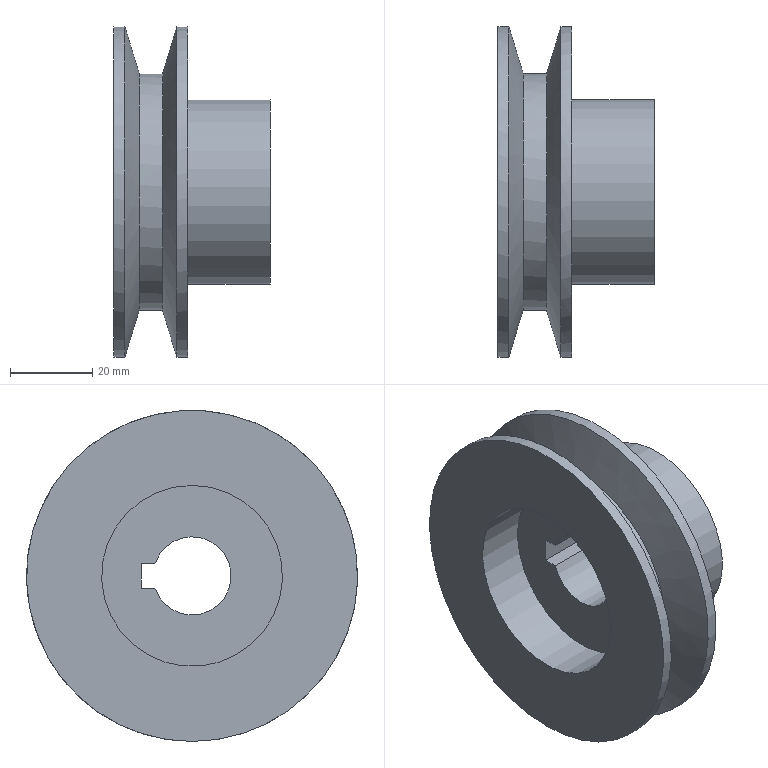Part | STEP file | Plain V-belt pulley_solid wheel_A75X16X1X38X45 | 1 solid | 15 faces | box 38 x 80.5 x 80.5 mm | volume 74057 mm3 | plane 7 | cylinder 6 | cone 2 | commonest cylinder face diameters 80.5 x2 19 x1 44 x1 45 x1 57.6 x1
STEP:
#1=CARTESIAN_POINT('',(0.,0.,0.));
#2=DIRECTION('',(0.,0.,1.));
#3=DIRECTION('',(1.,0.,0.));
#4=AXIS2_PLACEMENT_3D('',#1,#2,#3);
#5=CARTESIAN_POINT('',(12.,9.014,-3.));
#6=VERTEX_POINT('',#5);
#7=CARTESIAN_POINT('',(12.,12.3,-3.));
#8=VERTEX_POINT('',#7);
#9=CARTESIAN_POINT('',(12.,12.3,-3.));
#10=DIRECTION('',(0.,1.,0.));
#11=VECTOR('',#10,1.);
#12=LINE('',#9,#11);
#13=CARTESIAN_POINT('',(38.,12.3,-3.));
#14=DIRECTION('',(0.,0.,-1.));
#15=DIRECTION('',(0.,1.,0.));
#16=AXIS2_PLACEMENT_3D('',#13,#14,#15);
#17=PLANE('',#16);
#18=CARTESIAN_POINT('',(0.,-26.));
#19=DIRECTION('',(1.,0.));
#20=VECTOR('',#19,1.);
#21=LINE('',#18,#20);
#22=(GEOMETRIC_REPRESENTATION_CONTEXT(2)PARAMETRIC_REPRESENTATION_CONTEXT()REPRESENTATION_CONTEXT('',''));
#23=DEFINITIONAL_REPRESENTATION('',(#21),#22);
#24=PCURVE('',#17,#23);
#25=CARTESIAN_POINT('',(12.,0.,0.));
#26=DIRECTION('',(-1.,0.,0.));
#27=DIRECTION('',(0.,0.,1.));
#28=AXIS2_PLACEMENT_3D('',#25,#26,#27);
#29=PLANE('',#28);
#30=CARTESIAN_POINT('',(-3.,12.3));
#31=DIRECTION('',(0.,1.));
#32=VECTOR('',#31,1.);
#33=LINE('',#30,#32);
#34=(GEOMETRIC_REPRESENTATION_CONTEXT(2)PARAMETRIC_REPRESENTATION_CONTEXT()REPRESENTATION_CONTEXT('',''));
#35=DEFINITIONAL_REPRESENTATION('',(#33),#34);
#36=PCURVE('',#29,#35);
#37=SURFACE_CURVE('',#12,(#24,#36),.PCURVE_S1.);
#38=EDGE_CURVE('',#6,#8,#37,.T.);
#39=ORIENTED_EDGE('',*,*,#38,.F.);
#40=CARTESIAN_POINT('',(38.,9.014,-3.));
#41=VERTEX_POINT('',#40);
#42=CARTESIAN_POINT('',(38.,9.014,-3.));
#43=DIRECTION('',(-1.,0.,0.));
#44=VECTOR('',#43,1.);
#45=LINE('',#42,#44);
#46=CARTESIAN_POINT('',(-3.286,0.));
#47=DIRECTION('',(0.,-1.));
#48=VECTOR('',#47,1.);
#49=LINE('',#46,#48);
#50=(GEOMETRIC_REPRESENTATION_CONTEXT(2)PARAMETRIC_REPRESENTATION_CONTEXT()REPRESENTATION_CONTEXT('',''));
#51=DEFINITIONAL_REPRESENTATION('',(#49),#50);
#52=PCURVE('',#17,#51);
#53=CARTESIAN_POINT('',(38.,0.,0.));
#54=DIRECTION('',(-1.,0.,0.));
#55=DIRECTION('',(0.,0.,1.));
#56=AXIS2_PLACEMENT_3D('',#53,#54,#55);
#57=CYLINDRICAL_SURFACE('',#56,9.5);
#58=CARTESIAN_POINT('',(1.892,0.));
#59=DIRECTION('',(0.,1.));
#60=VECTOR('',#59,1.);
#61=LINE('',#58,#60);
#62=(GEOMETRIC_REPRESENTATION_CONTEXT(2)PARAMETRIC_REPRESENTATION_CONTEXT()REPRESENTATION_CONTEXT('',''));
#63=DEFINITIONAL_REPRESENTATION('',(#61),#62);
#64=PCURVE('',#57,#63);
#65=SURFACE_CURVE('',#45,(#52,#64),.PCURVE_S1.);
#66=EDGE_CURVE('',#41,#6,#65,.T.);
#67=ORIENTED_EDGE('',*,*,#66,.F.);
#68=CARTESIAN_POINT('',(38.,12.3,-3.));
#69=VERTEX_POINT('',#68);
#70=CARTESIAN_POINT('',(38.,12.3,-3.));
#71=DIRECTION('',(0.,-1.,0.));
#72=VECTOR('',#71,1.);
#73=LINE('',#70,#72);
#74=CARTESIAN_POINT('',(0.,0.));
#75=DIRECTION('',(-1.,0.));
#76=VECTOR('',#75,1.);
#77=LINE('',#74,#76);
#78=(GEOMETRIC_REPRESENTATION_CONTEXT(2)PARAMETRIC_REPRESENTATION_CONTEXT()REPRESENTATION_CONTEXT('',''));
#79=DEFINITIONAL_REPRESENTATION('',(#77),#78);
#80=PCURVE('',#17,#79);
#81=CARTESIAN_POINT('',(38.,15.25,0.));
#82=DIRECTION('',(1.,0.,0.));
#83=DIRECTION('',(0.,0.,-1.));
#84=AXIS2_PLACEMENT_3D('',#81,#82,#83);
#85=PLANE('',#84);
#86=CARTESIAN_POINT('',(3.,-2.95));
#87=DIRECTION('',(0.,-1.));
#88=VECTOR('',#87,1.);
#89=LINE('',#86,#88);
#90=(GEOMETRIC_REPRESENTATION_CONTEXT(2)PARAMETRIC_REPRESENTATION_CONTEXT()REPRESENTATION_CONTEXT('',''));
#91=DEFINITIONAL_REPRESENTATION('',(#89),#90);
#92=PCURVE('',#85,#91);
#93=SURFACE_CURVE('',#73,(#80,#92),.PCURVE_S1.);
#94=EDGE_CURVE('',#69,#41,#93,.T.);
#95=ORIENTED_EDGE('',*,*,#94,.F.);
#96=CARTESIAN_POINT('',(38.,12.3,-3.));
#97=DIRECTION('',(-1.,0.,0.));
#98=VECTOR('',#97,1.);
#99=LINE('',#96,#98);
#100=CARTESIAN_POINT('',(0.,0.));
#101=DIRECTION('',(0.,-1.));
#102=VECTOR('',#101,1.);
#103=LINE('',#100,#102);
#104=(GEOMETRIC_REPRESENTATION_CONTEXT(2)PARAMETRIC_REPRESENTATION_CONTEXT()REPRESENTATION_CONTEXT('',''));
#105=DEFINITIONAL_REPRESENTATION('',(#103),#104);
#106=PCURVE('',#17,#105);
#107=CARTESIAN_POINT('',(38.,12.3,-3.));
#108=DIRECTION('',(0.,1.,0.));
#109=DIRECTION('',(0.,0.,1.));
#110=AXIS2_PLACEMENT_3D('',#107,#108,#109);
#111=PLANE('',#110);
#112=CARTESIAN_POINT('',(0.,0.));
#113=DIRECTION('',(0.,-1.));
#114=VECTOR('',#113,1.);
#115=LINE('',#112,#114);
#116=(GEOMETRIC_REPRESENTATION_CONTEXT(2)PARAMETRIC_REPRESENTATION_CONTEXT()REPRESENTATION_CONTEXT('',''));
#117=DEFINITIONAL_REPRESENTATION('',(#115),#116);
#118=PCURVE('',#111,#117);
#119=SURFACE_CURVE('',#99,(#106,#118),.PCURVE_S1.);
#120=EDGE_CURVE('',#69,#8,#119,.T.);
#121=ORIENTED_EDGE('',*,*,#120,.T.);
#122=EDGE_LOOP('',(#39,#67,#95,#121));
#123=FACE_BOUND('',#122,.T.);
#124=ADVANCED_FACE('',(#123),#17,.F.);
#125=CARTESIAN_POINT('',(12.,12.3,3.));
#126=VERTEX_POINT('',#125);
#127=CARTESIAN_POINT('',(12.,12.3,-3.));
#128=DIRECTION('',(0.,0.,1.));
#129=VECTOR('',#128,1.);
#130=LINE('',#127,#129);
#131=CARTESIAN_POINT('',(0.,-26.));
#132=DIRECTION('',(1.,0.));
#133=VECTOR('',#132,1.);
#134=LINE('',#131,#133);
#135=(GEOMETRIC_REPRESENTATION_CONTEXT(2)PARAMETRIC_REPRESENTATION_CONTEXT()REPRESENTATION_CONTEXT('',''));
#136=DEFINITIONAL_REPRESENTATION('',(#134),#135);
#137=PCURVE('',#111,#136);
#138=CARTESIAN_POINT('',(-3.,12.3));
#139=DIRECTION('',(1.,0.));
#140=VECTOR('',#139,1.);
#141=LINE('',#138,#140);
#142=(GEOMETRIC_REPRESENTATION_CONTEXT(2)PARAMETRIC_REPRESENTATION_CONTEXT()REPRESENTATION_CONTEXT('',''));
#143=DEFINITIONAL_REPRESENTATION('',(#141),#142);
#144=PCURVE('',#29,#143);
#145=SURFACE_CURVE('',#130,(#137,#144),.PCURVE_S1.);
#146=EDGE_CURVE('',#8,#126,#145,.T.);
#147=ORIENTED_EDGE('',*,*,#146,.F.);
#148=ORIENTED_EDGE('',*,*,#120,.F.);
#149=CARTESIAN_POINT('',(38.,12.3,3.));
#150=VERTEX_POINT('',#149);
#151=CARTESIAN_POINT('',(38.,12.3,-3.));
#152=DIRECTION('',(0.,0.,-1.));
#153=VECTOR('',#152,1.);
#154=LINE('',#151,#153);
#155=CARTESIAN_POINT('',(0.,0.));
#156=DIRECTION('',(-1.,0.));
#157=VECTOR('',#156,1.);
#158=LINE('',#155,#157);
#159=(GEOMETRIC_REPRESENTATION_CONTEXT(2)PARAMETRIC_REPRESENTATION_CONTEXT()REPRESENTATION_CONTEXT('',''));
#160=DEFINITIONAL_REPRESENTATION('',(#158),#159);
#161=PCURVE('',#111,#160);
#162=CARTESIAN_POINT('',(3.,-2.95));
#163=DIRECTION('',(1.,0.));
#164=VECTOR('',#163,1.);
#165=LINE('',#162,#164);
#166=(GEOMETRIC_REPRESENTATION_CONTEXT(2)PARAMETRIC_REPRESENTATION_CONTEXT()REPRESENTATION_CONTEXT('',''));
#167=DEFINITIONAL_REPRESENTATION('',(#165),#166);
#168=PCURVE('',#85,#167);
#169=SURFACE_CURVE('',#154,(#161,#168),.PCURVE_S1.);
#170=EDGE_CURVE('',#150,#69,#169,.T.);
#171=ORIENTED_EDGE('',*,*,#170,.F.);
#172=CARTESIAN_POINT('',(38.,12.3,3.));
#173=DIRECTION('',(-1.,0.,0.));
#174=VECTOR('',#173,1.);
#175=LINE('',#172,#174);
#176=CARTESIAN_POINT('',(6.,0.));
#177=DIRECTION('',(0.,-1.));
#178=VECTOR('',#177,1.);
#179=LINE('',#176,#178);
#180=(GEOMETRIC_REPRESENTATION_CONTEXT(2)PARAMETRIC_REPRESENTATION_CONTEXT()REPRESENTATION_CONTEXT('',''));
#181=DEFINITIONAL_REPRESENTATION('',(#179),#180);
#182=PCURVE('',#111,#181);
#183=CARTESIAN_POINT('',(38.,12.3,3.));
#184=DIRECTION('',(0.,0.,1.));
#185=DIRECTION('',(1.,0.,0.));
#186=AXIS2_PLACEMENT_3D('',#183,#184,#185);
#187=PLANE('',#186);
#188=CARTESIAN_POINT('',(0.,0.));
#189=DIRECTION('',(-1.,0.));
#190=VECTOR('',#189,1.);
#191=LINE('',#188,#190);
#192=(GEOMETRIC_REPRESENTATION_CONTEXT(2)PARAMETRIC_REPRESENTATION_CONTEXT()REPRESENTATION_CONTEXT('',''));
#193=DEFINITIONAL_REPRESENTATION('',(#191),#192);
#194=PCURVE('',#187,#193);
#195=SURFACE_CURVE('',#175,(#182,#194),.PCURVE_S1.);
#196=EDGE_CURVE('',#150,#126,#195,.T.);
#197=ORIENTED_EDGE('',*,*,#196,.T.);
#198=EDGE_LOOP('',(#147,#148,#171,#197));
#199=FACE_BOUND('',#198,.T.);
#200=ADVANCED_FACE('',(#199),#111,.F.);
#201=CARTESIAN_POINT('',(12.,9.014,3.));
#202=VERTEX_POINT('',#201);
#203=CARTESIAN_POINT('',(12.,12.3,3.));
#204=DIRECTION('',(0.,-1.,0.));
#205=VECTOR('',#204,1.);
#206=LINE('',#203,#205);
#207=CARTESIAN_POINT('',(-26.,0.));
#208=DIRECTION('',(0.,-1.));
#209=VECTOR('',#208,1.);
#210=LINE('',#207,#209);
#211=(GEOMETRIC_REPRESENTATION_CONTEXT(2)PARAMETRIC_REPRESENTATION_CONTEXT()REPRESENTATION_CONTEXT('',''));
#212=DEFINITIONAL_REPRESENTATION('',(#210),#211);
#213=PCURVE('',#187,#212);
#214=CARTESIAN_POINT('',(3.,12.3));
#215=DIRECTION('',(0.,-1.));
#216=VECTOR('',#215,1.);
#217=LINE('',#214,#216);
#218=(GEOMETRIC_REPRESENTATION_CONTEXT(2)PARAMETRIC_REPRESENTATION_CONTEXT()REPRESENTATION_CONTEXT('',''));
#219=DEFINITIONAL_REPRESENTATION('',(#217),#218);
#220=PCURVE('',#29,#219);
#221=SURFACE_CURVE('',#206,(#213,#220),.PCURVE_S1.);
#222=EDGE_CURVE('',#126,#202,#221,.T.);
#223=ORIENTED_EDGE('',*,*,#222,.F.);
#224=ORIENTED_EDGE('',*,*,#196,.F.);
#225=CARTESIAN_POINT('',(38.,9.014,3.));
#226=VERTEX_POINT('',#225);
#227=CARTESIAN_POINT('',(38.,12.3,3.));
#228=DIRECTION('',(0.,1.,0.));
#229=VECTOR('',#228,1.);
#230=LINE('',#227,#229);
#231=CARTESIAN_POINT('',(0.,0.));
#232=DIRECTION('',(0.,1.));
#233=VECTOR('',#232,1.);
#234=LINE('',#231,#233);
#235=(GEOMETRIC_REPRESENTATION_CONTEXT(2)PARAMETRIC_REPRESENTATION_CONTEXT()REPRESENTATION_CONTEXT('',''));
#236=DEFINITIONAL_REPRESENTATION('',(#234),#235);
#237=PCURVE('',#187,#236);
#238=CARTESIAN_POINT('',(-3.,-2.95));
#239=DIRECTION('',(0.,1.));
#240=VECTOR('',#239,1.);
#241=LINE('',#238,#240);
#242=(GEOMETRIC_REPRESENTATION_CONTEXT(2)PARAMETRIC_REPRESENTATION_CONTEXT()REPRESENTATION_CONTEXT('',''));
#243=DEFINITIONAL_REPRESENTATION('',(#241),#242);
#244=PCURVE('',#85,#243);
#245=SURFACE_CURVE('',#230,(#237,#244),.PCURVE_S1.);
#246=EDGE_CURVE('',#226,#150,#245,.T.);
#247=ORIENTED_EDGE('',*,*,#246,.F.);
#248=CARTESIAN_POINT('',(38.,9.014,3.));
#249=DIRECTION('',(-1.,0.,0.));
#250=VECTOR('',#249,1.);
#251=LINE('',#248,#250);
#252=CARTESIAN_POINT('',(0.,-3.286));
#253=DIRECTION('',(-1.,0.));
#254=VECTOR('',#253,1.);
#255=LINE('',#252,#254);
#256=(GEOMETRIC_REPRESENTATION_CONTEXT(2)PARAMETRIC_REPRESENTATION_CONTEXT()REPRESENTATION_CONTEXT('',''));
#257=DEFINITIONAL_REPRESENTATION('',(#255),#256);
#258=PCURVE('',#187,#257);
#259=CARTESIAN_POINT('',(7.533,0.));
#260=DIRECTION('',(0.,1.));
#261=VECTOR('',#260,1.);
#262=LINE('',#259,#261);
#263=(GEOMETRIC_REPRESENTATION_CONTEXT(2)PARAMETRIC_REPRESENTATION_CONTEXT()REPRESENTATION_CONTEXT('',''));
#264=DEFINITIONAL_REPRESENTATION('',(#262),#263);
#265=PCURVE('',#57,#264);
#266=SURFACE_CURVE('',#251,(#258,#265),.PCURVE_S1.);
#267=EDGE_CURVE('',#226,#202,#266,.T.);
#268=ORIENTED_EDGE('',*,*,#267,.T.);
#269=EDGE_LOOP('',(#223,#224,#247,#268));
#270=FACE_BOUND('',#269,.T.);
#271=ADVANCED_FACE('',(#270),#187,.F.);
#272=ORIENTED_EDGE('',*,*,#66,.F.);
#273=CARTESIAN_POINT('',(38.,0.,0.));
#274=DIRECTION('',(-1.,0.,0.));
#275=DIRECTION('',(0.,0.,1.));
#276=AXIS2_PLACEMENT_3D('',#273,#274,#275);
#277=CIRCLE('',#276,9.5);
#278=CARTESIAN_POINT('',(0.,0.));
#279=DIRECTION('',(1.,0.));
#280=VECTOR('',#279,1.);
#281=LINE('',#278,#280);
#282=(GEOMETRIC_REPRESENTATION_CONTEXT(2)PARAMETRIC_REPRESENTATION_CONTEXT()REPRESENTATION_CONTEXT('',''));
#283=DEFINITIONAL_REPRESENTATION('',(#281),#282);
#284=PCURVE('',#57,#283);
#285=CARTESIAN_POINT('',(-9.5,-15.25));
#286=CARTESIAN_POINT('',(-9.5,1.204));
#287=CARTESIAN_POINT('',(4.75,-7.023));
#288=CARTESIAN_POINT('',(19.,-15.25));
#289=CARTESIAN_POINT('',(4.75,-23.477));
#290=CARTESIAN_POINT('',(-9.5,-31.704));
#291=CARTESIAN_POINT('',(-9.5,-15.25));
#292=(BOUNDED_CURVE()B_SPLINE_CURVE(2,(#285,#286,#287,#288,#289,#290,#291),.UNSPECIFIED.,.T.,.F.)B_SPLINE_CURVE_WITH_KNOTS((1,2,2,2,2,1),(-2.094,0.,2.094,4.189,6.283,8.378),.UNSPECIFIED.)CURVE()GEOMETRIC_REPRESENTATION_ITEM()RATIONAL_B_SPLINE_CURVE((1.,0.5,1.,0.5,1.,0.5,1.))REPRESENTATION_ITEM(''));
#293=(GEOMETRIC_REPRESENTATION_CONTEXT(2)PARAMETRIC_REPRESENTATION_CONTEXT()REPRESENTATION_CONTEXT('',''));
#294=DEFINITIONAL_REPRESENTATION('',(#292),#293);
#295=PCURVE('',#85,#294);
#296=SURFACE_CURVE('',#277,(#284,#295),.PCURVE_S1.);
#297=EDGE_CURVE('',#41,#226,#296,.T.);
#298=ORIENTED_EDGE('',*,*,#297,.T.);
#299=ORIENTED_EDGE('',*,*,#267,.T.);
#300=CARTESIAN_POINT('',(12.,0.,0.));
#301=DIRECTION('',(1.,0.,0.));
#302=DIRECTION('',(0.,0.,1.));
#303=AXIS2_PLACEMENT_3D('',#300,#301,#302);
#304=CIRCLE('',#303,9.5);
#305=CARTESIAN_POINT('',(12.566,26.));
#306=DIRECTION('',(-1.,0.));
#307=VECTOR('',#306,1.);
#308=LINE('',#305,#307);
#309=(GEOMETRIC_REPRESENTATION_CONTEXT(2)PARAMETRIC_REPRESENTATION_CONTEXT()REPRESENTATION_CONTEXT('',''));
#310=DEFINITIONAL_REPRESENTATION('',(#308),#309);
#311=PCURVE('',#57,#310);
#312=CARTESIAN_POINT('',(9.5,0.));
#313=CARTESIAN_POINT('',(9.5,-16.454));
#314=CARTESIAN_POINT('',(-4.75,-8.227));
#315=CARTESIAN_POINT('',(-19.,0.));
#316=CARTESIAN_POINT('',(-4.75,8.227));
#317=CARTESIAN_POINT('',(9.5,16.454));
#318=CARTESIAN_POINT('',(9.5,0.));
#319=(BOUNDED_CURVE()B_SPLINE_CURVE(2,(#312,#313,#314,#315,#316,#317,#318),.UNSPECIFIED.,.T.,.F.)B_SPLINE_CURVE_WITH_KNOTS((1,2,2,2,2,1),(-2.094,0.,2.094,4.189,6.283,8.378),.UNSPECIFIED.)CURVE()GEOMETRIC_REPRESENTATION_ITEM()RATIONAL_B_SPLINE_CURVE((1.,0.5,1.,0.5,1.,0.5,1.))REPRESENTATION_ITEM(''));
#320=(GEOMETRIC_REPRESENTATION_CONTEXT(2)PARAMETRIC_REPRESENTATION_CONTEXT()REPRESENTATION_CONTEXT('',''));
#321=DEFINITIONAL_REPRESENTATION('',(#319),#320);
#322=PCURVE('',#29,#321);
#323=SURFACE_CURVE('',#304,(#311,#322),.PCURVE_S1.);
#324=EDGE_CURVE('',#202,#6,#323,.T.);
#325=ORIENTED_EDGE('',*,*,#324,.T.);
#326=EDGE_LOOP('',(#272,#298,#299,#325));
#327=FACE_BOUND('',#326,.F.);
#328=ADVANCED_FACE('',(#327),#57,.F.);
#329=CARTESIAN_POINT('',(0.,0.,22.));
#330=VERTEX_POINT('',#329);
#331=CARTESIAN_POINT('',(0.,0.,0.));
#332=DIRECTION('',(-1.,0.,0.));
#333=DIRECTION('',(0.,0.,1.));
#334=AXIS2_PLACEMENT_3D('',#331,#332,#333);
#335=CIRCLE('',#334,22.);
#336=CARTESIAN_POINT('',(0.,31.375,0.));
#337=DIRECTION('',(-1.,0.,0.));
#338=DIRECTION('',(0.,0.,1.));
#339=AXIS2_PLACEMENT_3D('',#336,#337,#338);
#340=PLANE('',#339);
#341=CARTESIAN_POINT('',(0.,-31.375));
#342=DIRECTION('',(1.,0.));
#343=AXIS2_PLACEMENT_2D('',#341,#342);
#344=CIRCLE('',#343,22.);
#345=(GEOMETRIC_REPRESENTATION_CONTEXT(2)PARAMETRIC_REPRESENTATION_CONTEXT()REPRESENTATION_CONTEXT('',''));
#346=DEFINITIONAL_REPRESENTATION('',(#344),#345);
#347=PCURVE('',#340,#346);
#348=CARTESIAN_POINT('',(12.,0.,0.));
#349=DIRECTION('',(-1.,0.,0.));
#350=DIRECTION('',(0.,0.,1.));
#351=AXIS2_PLACEMENT_3D('',#348,#349,#350);
#352=CYLINDRICAL_SURFACE('',#351,22.);
#353=CARTESIAN_POINT('',(0.,12.));
#354=DIRECTION('',(1.,0.));
#355=VECTOR('',#354,1.);
#356=LINE('',#353,#355);
#357=(GEOMETRIC_REPRESENTATION_CONTEXT(2)PARAMETRIC_REPRESENTATION_CONTEXT()REPRESENTATION_CONTEXT('',''));
#358=DEFINITIONAL_REPRESENTATION('',(#356),#357);
#359=PCURVE('',#352,#358);
#360=SURFACE_CURVE('',#335,(#347,#359),.PCURVE_S1.);
#361=EDGE_CURVE('',#330,#330,#360,.T.);
#362=ORIENTED_EDGE('',*,*,#361,.F.);
#363=EDGE_LOOP('',(#362));
#364=FACE_BOUND('',#363,.T.);
#365=CARTESIAN_POINT('',(0.,0.,-40.25));
#366=VERTEX_POINT('',#365);
#367=CARTESIAN_POINT('',(0.,0.,0.));
#368=DIRECTION('',(-1.,0.,0.));
#369=DIRECTION('',(0.,0.,-1.));
#370=AXIS2_PLACEMENT_3D('',#367,#368,#369);
#371=CIRCLE('',#370,40.25);
#372=CARTESIAN_POINT('',(0.,-31.375));
#373=DIRECTION('',(-1.,0.));
#374=AXIS2_PLACEMENT_2D('',#372,#373);
#375=CIRCLE('',#374,40.25);
#376=(GEOMETRIC_REPRESENTATION_CONTEXT(2)PARAMETRIC_REPRESENTATION_CONTEXT()REPRESENTATION_CONTEXT('',''));
#377=DEFINITIONAL_REPRESENTATION('',(#375),#376);
#378=PCURVE('',#340,#377);
#379=CARTESIAN_POINT('',(9.,0.,0.));
#380=DIRECTION('',(1.,0.,0.));
#381=DIRECTION('',(0.,0.,-1.));
#382=AXIS2_PLACEMENT_3D('',#379,#380,#381);
#383=CYLINDRICAL_SURFACE('',#382,40.25);
#384=CARTESIAN_POINT('',(6.283,-9.));
#385=DIRECTION('',(-1.,0.));
#386=VECTOR('',#385,1.);
#387=LINE('',#384,#386);
#388=(GEOMETRIC_REPRESENTATION_CONTEXT(2)PARAMETRIC_REPRESENTATION_CONTEXT()REPRESENTATION_CONTEXT('',''));
#389=DEFINITIONAL_REPRESENTATION('',(#387),#388);
#390=PCURVE('',#383,#389);
#391=SURFACE_CURVE('',#371,(#378,#390),.PCURVE_S1.);
#392=EDGE_CURVE('',#366,#366,#391,.T.);
#393=ORIENTED_EDGE('',*,*,#392,.T.);
#394=EDGE_LOOP('',(#393));
#395=FACE_BOUND('',#394,.T.);
#396=ADVANCED_FACE('',(#364,#395),#340,.T.);
#397=CARTESIAN_POINT('',(2.659,0.,-40.25));
#398=VERTEX_POINT('',#397);
#399=CARTESIAN_POINT('',(2.659,40.25,0.));
#400=VERTEX_POINT('',#399);
#401=CARTESIAN_POINT('',(2.659,0.,0.));
#402=DIRECTION('',(-1.,0.,0.));
#403=DIRECTION('',(0.,0.,-1.));
#404=AXIS2_PLACEMENT_3D('',#401,#402,#403);
#405=CIRCLE('',#404,40.25);
#406=CARTESIAN_POINT('',(6.283,-6.341));
#407=DIRECTION('',(-1.,0.));
#408=VECTOR('',#407,1.);
#409=LINE('',#406,#408);
#410=(GEOMETRIC_REPRESENTATION_CONTEXT(2)PARAMETRIC_REPRESENTATION_CONTEXT()REPRESENTATION_CONTEXT('',''));
#411=DEFINITIONAL_REPRESENTATION('',(#409),#410);
#412=PCURVE('',#383,#411);
#413=CARTESIAN_POINT('',(2.659,0.,0.));
#414=DIRECTION('',(-1.,0.,0.));
#415=DIRECTION('',(0.,0.,1.));
#416=AXIS2_PLACEMENT_3D('',#413,#414,#415);
#417=CONICAL_SURFACE('',#416,40.25,1.274);
#418=CARTESIAN_POINT('',(3.142,0.));
#419=DIRECTION('',(1.,0.));
#420=VECTOR('',#419,1.);
#421=LINE('',#418,#420);
#422=(GEOMETRIC_REPRESENTATION_CONTEXT(2)PARAMETRIC_REPRESENTATION_CONTEXT()REPRESENTATION_CONTEXT('',''));
#423=DEFINITIONAL_REPRESENTATION('',(#421),#422);
#424=PCURVE('',#417,#423);
#425=SURFACE_CURVE('',#405,(#412,#424),.PCURVE_S1.);
#426=EDGE_CURVE('',#398,#400,#425,.T.);
#427=ORIENTED_EDGE('',*,*,#426,.T.);
#428=CARTESIAN_POINT('',(2.659,0.,0.));
#429=DIRECTION('',(-1.,0.,0.));
#430=DIRECTION('',(0.,0.,-1.));
#431=AXIS2_PLACEMENT_3D('',#428,#429,#430);
#432=CIRCLE('',#431,40.25);
#433=CARTESIAN_POINT('',(6.283,-6.341));
#434=DIRECTION('',(-1.,0.));
#435=VECTOR('',#434,1.);
#436=LINE('',#433,#435);
#437=(GEOMETRIC_REPRESENTATION_CONTEXT(2)PARAMETRIC_REPRESENTATION_CONTEXT()REPRESENTATION_CONTEXT('',''));
#438=DEFINITIONAL_REPRESENTATION('',(#436),#437);
#439=PCURVE('',#383,#438);
#440=CARTESIAN_POINT('',(-3.142,0.));
#441=DIRECTION('',(1.,0.));
#442=VECTOR('',#441,1.);
#443=LINE('',#440,#442);
#444=(GEOMETRIC_REPRESENTATION_CONTEXT(2)PARAMETRIC_REPRESENTATION_CONTEXT()REPRESENTATION_CONTEXT('',''));
#445=DEFINITIONAL_REPRESENTATION('',(#443),#444);
#446=PCURVE('',#417,#445);
#447=SURFACE_CURVE('',#432,(#439,#446),.PCURVE_S1.);
#448=EDGE_CURVE('',#400,#398,#447,.T.);
#449=ORIENTED_EDGE('',*,*,#448,.T.);
#450=CARTESIAN_POINT('',(0.,0.,-40.25));
#451=CARTESIAN_POINT('',(2.659,0.,-40.25));
#452=B_SPLINE_CURVE_WITH_KNOTS('',1,(#450,#451),.UNSPECIFIED.,.F.,.F.,(2,2),(-9.,-6.341),.PIECEWISE_BEZIER_KNOTS.);
#453=CARTESIAN_POINT('',(0.,0.));
#454=DIRECTION('',(0.,1.));
#455=VECTOR('',#454,1.);
#456=LINE('',#453,#455);
#457=(GEOMETRIC_REPRESENTATION_CONTEXT(2)PARAMETRIC_REPRESENTATION_CONTEXT()REPRESENTATION_CONTEXT('',''));
#458=DEFINITIONAL_REPRESENTATION('',(#456),#457);
#459=PCURVE('',#383,#458);
#460=CARTESIAN_POINT('',(6.283,0.));
#461=DIRECTION('',(0.,1.));
#462=VECTOR('',#461,1.);
#463=LINE('',#460,#462);
#464=(GEOMETRIC_REPRESENTATION_CONTEXT(2)PARAMETRIC_REPRESENTATION_CONTEXT()REPRESENTATION_CONTEXT('',''));
#465=DEFINITIONAL_REPRESENTATION('',(#463),#464);
#466=PCURVE('',#383,#465);
#467=SEAM_CURVE('',#452,(#459,#466),.PCURVE_S1.);
#468=EDGE_CURVE('',#366,#398,#467,.T.);
#469=ORIENTED_EDGE('',*,*,#468,.F.);
#470=ORIENTED_EDGE('',*,*,#392,.F.);
#471=ORIENTED_EDGE('',*,*,#468,.T.);
#472=EDGE_LOOP('',(#427,#449,#469,#470,#471));
#473=FACE_BOUND('',#472,.T.);
#474=ADVANCED_FACE('',(#473),#383,.T.);
#475=CARTESIAN_POINT('',(6.16,28.8,0.));
#476=VERTEX_POINT('',#475);
#477=CARTESIAN_POINT('',(6.16,0.,-28.8));
#478=VERTEX_POINT('',#477);
#479=CARTESIAN_POINT('',(6.16,0.,0.));
#480=DIRECTION('',(-1.,0.,0.));
#481=DIRECTION('',(0.,1.,0.));
#482=AXIS2_PLACEMENT_3D('',#479,#480,#481);
#483=CIRCLE('',#482,28.8);
#484=CARTESIAN_POINT('',(1.571,-3.501));
#485=DIRECTION('',(1.,0.));
#486=VECTOR('',#485,1.);
#487=LINE('',#484,#486);
#488=(GEOMETRIC_REPRESENTATION_CONTEXT(2)PARAMETRIC_REPRESENTATION_CONTEXT()REPRESENTATION_CONTEXT('',''));
#489=DEFINITIONAL_REPRESENTATION('',(#487),#488);
#490=PCURVE('',#417,#489);
#491=CARTESIAN_POINT('',(9.,0.,0.));
#492=DIRECTION('',(1.,0.,0.));
#493=DIRECTION('',(0.,0.,-1.));
#494=AXIS2_PLACEMENT_3D('',#491,#492,#493);
#495=CYLINDRICAL_SURFACE('',#494,28.8);
#496=CARTESIAN_POINT('',(1.571,-2.84));
#497=DIRECTION('',(-1.,0.));
#498=VECTOR('',#497,1.);
#499=LINE('',#496,#498);
#500=(GEOMETRIC_REPRESENTATION_CONTEXT(2)PARAMETRIC_REPRESENTATION_CONTEXT()REPRESENTATION_CONTEXT('',''));
#501=DEFINITIONAL_REPRESENTATION('',(#499),#500);
#502=PCURVE('',#495,#501);
#503=SURFACE_CURVE('',#483,(#490,#502),.PCURVE_S1.);
#504=EDGE_CURVE('',#476,#478,#503,.T.);
#505=ORIENTED_EDGE('',*,*,#504,.T.);
#506=CARTESIAN_POINT('',(6.16,0.,0.));
#507=DIRECTION('',(-1.,0.,0.));
#508=DIRECTION('',(0.,1.,0.));
#509=AXIS2_PLACEMENT_3D('',#506,#507,#508);
#510=CIRCLE('',#509,28.8);
#511=CARTESIAN_POINT('',(1.571,-3.501));
#512=DIRECTION('',(1.,0.));
#513=VECTOR('',#512,1.);
#514=LINE('',#511,#513);
#515=(GEOMETRIC_REPRESENTATION_CONTEXT(2)PARAMETRIC_REPRESENTATION_CONTEXT()REPRESENTATION_CONTEXT('',''));
#516=DEFINITIONAL_REPRESENTATION('',(#514),#515);
#517=PCURVE('',#417,#516);
#518=CARTESIAN_POINT('',(7.854,-2.84));
#519=DIRECTION('',(-1.,0.));
#520=VECTOR('',#519,1.);
#521=LINE('',#518,#520);
#522=(GEOMETRIC_REPRESENTATION_CONTEXT(2)PARAMETRIC_REPRESENTATION_CONTEXT()REPRESENTATION_CONTEXT('',''));
#523=DEFINITIONAL_REPRESENTATION('',(#521),#522);
#524=PCURVE('',#495,#523);
#525=SURFACE_CURVE('',#510,(#517,#524),.PCURVE_S1.);
#526=EDGE_CURVE('',#478,#476,#525,.T.);
#527=ORIENTED_EDGE('',*,*,#526,.T.);
#528=CARTESIAN_POINT('',(6.16,28.8,0.));
#529=CARTESIAN_POINT('',(2.659,40.25,0.));
#530=B_SPLINE_CURVE_WITH_KNOTS('',1,(#528,#529),.UNSPECIFIED.,.F.,.F.,(2,2),(-11.973,0.),.PIECEWISE_BEZIER_KNOTS.);
#531=CARTESIAN_POINT('',(7.854,0.));
#532=DIRECTION('',(0.,1.));
#533=VECTOR('',#532,1.);
#534=LINE('',#531,#533);
#535=(GEOMETRIC_REPRESENTATION_CONTEXT(2)PARAMETRIC_REPRESENTATION_CONTEXT()REPRESENTATION_CONTEXT('',''));
#536=DEFINITIONAL_REPRESENTATION('',(#534),#535);
#537=PCURVE('',#417,#536);
#538=CARTESIAN_POINT('',(1.571,0.));
#539=DIRECTION('',(0.,1.));
#540=VECTOR('',#539,1.);
#541=LINE('',#538,#540);
#542=(GEOMETRIC_REPRESENTATION_CONTEXT(2)PARAMETRIC_REPRESENTATION_CONTEXT()REPRESENTATION_CONTEXT('',''));
#543=DEFINITIONAL_REPRESENTATION('',(#541),#542);
#544=PCURVE('',#417,#543);
#545=SEAM_CURVE('',#530,(#537,#544),.PCURVE_S1.);
#546=EDGE_CURVE('',#476,#400,#545,.T.);
#547=ORIENTED_EDGE('',*,*,#546,.T.);
#548=ORIENTED_EDGE('',*,*,#426,.F.);
#549=ORIENTED_EDGE('',*,*,#448,.F.);
#550=ORIENTED_EDGE('',*,*,#546,.F.);
#551=EDGE_LOOP('',(#505,#527,#547,#548,#549,#550));
#552=FACE_BOUND('',#551,.T.);
#553=ADVANCED_FACE('',(#552),#417,.T.);
#554=CARTESIAN_POINT('',(11.84,0.,-28.8));
#555=VERTEX_POINT('',#554);
#556=CARTESIAN_POINT('',(11.84,0.,0.));
#557=DIRECTION('',(-1.,0.,0.));
#558=DIRECTION('',(0.,0.,-1.));
#559=AXIS2_PLACEMENT_3D('',#556,#557,#558);
#560=CIRCLE('',#559,28.8);
#561=CARTESIAN_POINT('',(6.283,2.84));
#562=DIRECTION('',(-1.,0.));
#563=VECTOR('',#562,1.);
#564=LINE('',#561,#563);
#565=(GEOMETRIC_REPRESENTATION_CONTEXT(2)PARAMETRIC_REPRESENTATION_CONTEXT()REPRESENTATION_CONTEXT('',''));
#566=DEFINITIONAL_REPRESENTATION('',(#564),#565);
#567=PCURVE('',#495,#566);
#568=CARTESIAN_POINT('',(15.341,0.,0.));
#569=DIRECTION('',(1.,0.,0.));
#570=DIRECTION('',(0.,0.,-1.));
#571=AXIS2_PLACEMENT_3D('',#568,#569,#570);
#572=CONICAL_SURFACE('',#571,40.25,1.274);
#573=CARTESIAN_POINT('',(6.283,-3.501));
#574=DIRECTION('',(-1.,0.));
#575=VECTOR('',#574,1.);
#576=LINE('',#573,#575);
#577=(GEOMETRIC_REPRESENTATION_CONTEXT(2)PARAMETRIC_REPRESENTATION_CONTEXT()REPRESENTATION_CONTEXT('',''));
#578=DEFINITIONAL_REPRESENTATION('',(#576),#577);
#579=PCURVE('',#572,#578);
#580=SURFACE_CURVE('',#560,(#567,#579),.PCURVE_S1.);
#581=EDGE_CURVE('',#555,#555,#580,.T.);
#582=ORIENTED_EDGE('',*,*,#581,.T.);
#583=CARTESIAN_POINT('',(6.16,0.,-28.8));
#584=CARTESIAN_POINT('',(11.84,0.,-28.8));
#585=B_SPLINE_CURVE_WITH_KNOTS('',1,(#583,#584),.UNSPECIFIED.,.F.,.F.,(2,2),(-2.84,2.84),.PIECEWISE_BEZIER_KNOTS.);
#586=CARTESIAN_POINT('',(0.,0.));
#587=DIRECTION('',(0.,1.));
#588=VECTOR('',#587,1.);
#589=LINE('',#586,#588);
#590=(GEOMETRIC_REPRESENTATION_CONTEXT(2)PARAMETRIC_REPRESENTATION_CONTEXT()REPRESENTATION_CONTEXT('',''));
#591=DEFINITIONAL_REPRESENTATION('',(#589),#590);
#592=PCURVE('',#495,#591);
#593=CARTESIAN_POINT('',(6.283,0.));
#594=DIRECTION('',(0.,1.));
#595=VECTOR('',#594,1.);
#596=LINE('',#593,#595);
#597=(GEOMETRIC_REPRESENTATION_CONTEXT(2)PARAMETRIC_REPRESENTATION_CONTEXT()REPRESENTATION_CONTEXT('',''));
#598=DEFINITIONAL_REPRESENTATION('',(#596),#597);
#599=PCURVE('',#495,#598);
#600=SEAM_CURVE('',#585,(#592,#599),.PCURVE_S1.);
#601=EDGE_CURVE('',#478,#555,#600,.T.);
#602=ORIENTED_EDGE('',*,*,#601,.F.);
#603=ORIENTED_EDGE('',*,*,#504,.F.);
#604=ORIENTED_EDGE('',*,*,#526,.F.);
#605=ORIENTED_EDGE('',*,*,#601,.T.);
#606=EDGE_LOOP('',(#582,#602,#603,#604,#605));
#607=FACE_BOUND('',#606,.T.);
#608=ADVANCED_FACE('',(#607),#495,.T.);
#609=ORIENTED_EDGE('',*,*,#94,.T.);
#610=ORIENTED_EDGE('',*,*,#297,.T.);
#611=ORIENTED_EDGE('',*,*,#246,.T.);
#612=ORIENTED_EDGE('',*,*,#170,.T.);
#613=EDGE_LOOP('',(#609,#610,#611,#612));
#614=FACE_BOUND('',#613,.T.);
#615=CARTESIAN_POINT('',(38.,0.,-22.5));
#616=VERTEX_POINT('',#615);
#617=CARTESIAN_POINT('',(38.,0.,0.));
#618=DIRECTION('',(1.,0.,0.));
#619=DIRECTION('',(0.,0.,-1.));
#620=AXIS2_PLACEMENT_3D('',#617,#618,#619);
#621=CIRCLE('',#620,22.5);
#622=CARTESIAN_POINT('',(0.,-15.25));
#623=DIRECTION('',(1.,0.));
#624=AXIS2_PLACEMENT_2D('',#622,#623);
#625=CIRCLE('',#624,22.5);
#626=(GEOMETRIC_REPRESENTATION_CONTEXT(2)PARAMETRIC_REPRESENTATION_CONTEXT()REPRESENTATION_CONTEXT('',''));
#627=DEFINITIONAL_REPRESENTATION('',(#625),#626);
#628=PCURVE('',#85,#627);
#629=CARTESIAN_POINT('',(19.,0.,0.));
#630=DIRECTION('',(1.,0.,0.));
#631=DIRECTION('',(0.,0.,-1.));
#632=AXIS2_PLACEMENT_3D('',#629,#630,#631);
#633=CYLINDRICAL_SURFACE('',#632,22.5);
#634=CARTESIAN_POINT('',(0.,19.));
#635=DIRECTION('',(1.,0.));
#636=VECTOR('',#635,1.);
#637=LINE('',#634,#636);
#638=(GEOMETRIC_REPRESENTATION_CONTEXT(2)PARAMETRIC_REPRESENTATION_CONTEXT()REPRESENTATION_CONTEXT('',''));
#639=DEFINITIONAL_REPRESENTATION('',(#637),#638);
#640=PCURVE('',#633,#639);
#641=SURFACE_CURVE('',#621,(#628,#640),.PCURVE_S1.);
#642=EDGE_CURVE('',#616,#616,#641,.T.);
#643=ORIENTED_EDGE('',*,*,#642,.T.);
#644=EDGE_LOOP('',(#643));
#645=FACE_BOUND('',#644,.T.);
#646=ADVANCED_FACE('',(#614,#645),#85,.T.);
#647=CARTESIAN_POINT('',(15.341,40.25,0.));
#648=VERTEX_POINT('',#647);
#649=CARTESIAN_POINT('',(15.341,0.,-40.25));
#650=VERTEX_POINT('',#649);
#651=CARTESIAN_POINT('',(15.341,0.,0.));
#652=DIRECTION('',(-1.,0.,0.));
#653=DIRECTION('',(0.,1.,0.));
#654=AXIS2_PLACEMENT_3D('',#651,#652,#653);
#655=CIRCLE('',#654,40.25);
#656=CARTESIAN_POINT('',(1.571,0.));
#657=DIRECTION('',(-1.,0.));
#658=VECTOR('',#657,1.);
#659=LINE('',#656,#658);
#660=(GEOMETRIC_REPRESENTATION_CONTEXT(2)PARAMETRIC_REPRESENTATION_CONTEXT()REPRESENTATION_CONTEXT('',''));
#661=DEFINITIONAL_REPRESENTATION('',(#659),#660);
#662=PCURVE('',#572,#661);
#663=CARTESIAN_POINT('',(9.,0.,0.));
#664=DIRECTION('',(1.,0.,0.));
#665=DIRECTION('',(0.,0.,-1.));
#666=AXIS2_PLACEMENT_3D('',#663,#664,#665);
#667=CYLINDRICAL_SURFACE('',#666,40.25);
#668=CARTESIAN_POINT('',(1.571,6.341));
#669=DIRECTION('',(-1.,0.));
#670=VECTOR('',#669,1.);
#671=LINE('',#668,#670);
#672=(GEOMETRIC_REPRESENTATION_CONTEXT(2)PARAMETRIC_REPRESENTATION_CONTEXT()REPRESENTATION_CONTEXT('',''));
#673=DEFINITIONAL_REPRESENTATION('',(#671),#672);
#674=PCURVE('',#667,#673);
#675=SURFACE_CURVE('',#655,(#662,#674),.PCURVE_S1.);
#676=EDGE_CURVE('',#648,#650,#675,.T.);
#677=ORIENTED_EDGE('',*,*,#676,.T.);
#678=CARTESIAN_POINT('',(11.84,0.,-28.8));
#679=CARTESIAN_POINT('',(15.341,0.,-40.25));
#680=B_SPLINE_CURVE_WITH_KNOTS('',1,(#678,#679),.UNSPECIFIED.,.F.,.F.,(2,2),(-11.973,0.),.PIECEWISE_BEZIER_KNOTS.);
#681=CARTESIAN_POINT('',(0.,0.));
#682=DIRECTION('',(0.,1.));
#683=VECTOR('',#682,1.);
#684=LINE('',#681,#683);
#685=(GEOMETRIC_REPRESENTATION_CONTEXT(2)PARAMETRIC_REPRESENTATION_CONTEXT()REPRESENTATION_CONTEXT('',''));
#686=DEFINITIONAL_REPRESENTATION('',(#684),#685);
#687=PCURVE('',#572,#686);
#688=CARTESIAN_POINT('',(6.283,0.));
#689=DIRECTION('',(0.,1.));
#690=VECTOR('',#689,1.);
#691=LINE('',#688,#690);
#692=(GEOMETRIC_REPRESENTATION_CONTEXT(2)PARAMETRIC_REPRESENTATION_CONTEXT()REPRESENTATION_CONTEXT('',''));
#693=DEFINITIONAL_REPRESENTATION('',(#691),#692);
#694=PCURVE('',#572,#693);
#695=SEAM_CURVE('',#680,(#687,#694),.PCURVE_S1.);
#696=EDGE_CURVE('',#555,#650,#695,.T.);
#697=ORIENTED_EDGE('',*,*,#696,.F.);
#698=ORIENTED_EDGE('',*,*,#581,.F.);
#699=ORIENTED_EDGE('',*,*,#696,.T.);
#700=CARTESIAN_POINT('',(15.341,0.,0.));
#701=DIRECTION('',(-1.,0.,0.));
#702=DIRECTION('',(0.,1.,0.));
#703=AXIS2_PLACEMENT_3D('',#700,#701,#702);
#704=CIRCLE('',#703,40.25);
#705=CARTESIAN_POINT('',(7.854,0.));
#706=DIRECTION('',(-1.,0.));
#707=VECTOR('',#706,1.);
#708=LINE('',#705,#707);
#709=(GEOMETRIC_REPRESENTATION_CONTEXT(2)PARAMETRIC_REPRESENTATION_CONTEXT()REPRESENTATION_CONTEXT('',''));
#710=DEFINITIONAL_REPRESENTATION('',(#708),#709);
#711=PCURVE('',#572,#710);
#712=CARTESIAN_POINT('',(7.854,6.341));
#713=DIRECTION('',(-1.,0.));
#714=VECTOR('',#713,1.);
#715=LINE('',#712,#714);
#716=(GEOMETRIC_REPRESENTATION_CONTEXT(2)PARAMETRIC_REPRESENTATION_CONTEXT()REPRESENTATION_CONTEXT('',''));
#717=DEFINITIONAL_REPRESENTATION('',(#715),#716);
#718=PCURVE('',#667,#717);
#719=SURFACE_CURVE('',#704,(#711,#718),.PCURVE_S1.);
#720=EDGE_CURVE('',#650,#648,#719,.T.);
#721=ORIENTED_EDGE('',*,*,#720,.T.);
#722=EDGE_LOOP('',(#677,#697,#698,#699,#721));
#723=FACE_BOUND('',#722,.T.);
#724=ADVANCED_FACE('',(#723),#572,.T.);
#725=ORIENTED_EDGE('',*,*,#642,.F.);
#726=CARTESIAN_POINT('',(18.,0.,-22.5));
#727=VERTEX_POINT('',#726);
#728=CARTESIAN_POINT('',(18.,0.,-22.5));
#729=CARTESIAN_POINT('',(38.,0.,-22.5));
#730=B_SPLINE_CURVE_WITH_KNOTS('',1,(#728,#729),.UNSPECIFIED.,.F.,.F.,(2,2),(-1.,19.),.PIECEWISE_BEZIER_KNOTS.);
#731=CARTESIAN_POINT('',(0.,0.));
#732=DIRECTION('',(0.,1.));
#733=VECTOR('',#732,1.);
#734=LINE('',#731,#733);
#735=(GEOMETRIC_REPRESENTATION_CONTEXT(2)PARAMETRIC_REPRESENTATION_CONTEXT()REPRESENTATION_CONTEXT('',''));
#736=DEFINITIONAL_REPRESENTATION('',(#734),#735);
#737=PCURVE('',#633,#736);
#738=CARTESIAN_POINT('',(6.283,0.));
#739=DIRECTION('',(0.,1.));
#740=VECTOR('',#739,1.);
#741=LINE('',#738,#740);
#742=(GEOMETRIC_REPRESENTATION_CONTEXT(2)PARAMETRIC_REPRESENTATION_CONTEXT()REPRESENTATION_CONTEXT('',''));
#743=DEFINITIONAL_REPRESENTATION('',(#741),#742);
#744=PCURVE('',#633,#743);
#745=SEAM_CURVE('',#730,(#737,#744),.PCURVE_S1.);
#746=EDGE_CURVE('',#727,#616,#745,.T.);
#747=ORIENTED_EDGE('',*,*,#746,.F.);
#748=CARTESIAN_POINT('',(18.,0.,0.));
#749=DIRECTION('',(1.,0.,0.));
#750=DIRECTION('',(0.,0.,-1.));
#751=AXIS2_PLACEMENT_3D('',#748,#749,#750);
#752=CIRCLE('',#751,22.5);
#753=CARTESIAN_POINT('',(0.,-1.));
#754=DIRECTION('',(1.,0.));
#755=VECTOR('',#754,1.);
#756=LINE('',#753,#755);
#757=(GEOMETRIC_REPRESENTATION_CONTEXT(2)PARAMETRIC_REPRESENTATION_CONTEXT()REPRESENTATION_CONTEXT('',''));
#758=DEFINITIONAL_REPRESENTATION('',(#756),#757);
#759=PCURVE('',#633,#758);
#760=CARTESIAN_POINT('',(18.,31.375,0.));
#761=DIRECTION('',(1.,0.,0.));
#762=DIRECTION('',(0.,0.,-1.));
#763=AXIS2_PLACEMENT_3D('',#760,#761,#762);
#764=PLANE('',#763);
#765=CARTESIAN_POINT('',(0.,-31.375));
#766=DIRECTION('',(1.,0.));
#767=AXIS2_PLACEMENT_2D('',#765,#766);
#768=CIRCLE('',#767,22.5);
#769=(GEOMETRIC_REPRESENTATION_CONTEXT(2)PARAMETRIC_REPRESENTATION_CONTEXT()REPRESENTATION_CONTEXT('',''));
#770=DEFINITIONAL_REPRESENTATION('',(#768),#769);
#771=PCURVE('',#764,#770);
#772=SURFACE_CURVE('',#752,(#759,#771),.PCURVE_S1.);
#773=EDGE_CURVE('',#727,#727,#772,.T.);
#774=ORIENTED_EDGE('',*,*,#773,.T.);
#775=ORIENTED_EDGE('',*,*,#746,.T.);
#776=EDGE_LOOP('',(#725,#747,#774,#775));
#777=FACE_BOUND('',#776,.T.);
#778=ADVANCED_FACE('',(#777),#633,.T.);
#779=CARTESIAN_POINT('',(18.,0.,-40.25));
#780=VERTEX_POINT('',#779);
#781=CARTESIAN_POINT('',(18.,0.,0.));
#782=DIRECTION('',(-1.,0.,0.));
#783=DIRECTION('',(0.,0.,-1.));
#784=AXIS2_PLACEMENT_3D('',#781,#782,#783);
#785=CIRCLE('',#784,40.25);
#786=CARTESIAN_POINT('',(6.283,9.));
#787=DIRECTION('',(-1.,0.));
#788=VECTOR('',#787,1.);
#789=LINE('',#786,#788);
#790=(GEOMETRIC_REPRESENTATION_CONTEXT(2)PARAMETRIC_REPRESENTATION_CONTEXT()REPRESENTATION_CONTEXT('',''));
#791=DEFINITIONAL_REPRESENTATION('',(#789),#790);
#792=PCURVE('',#667,#791);
#793=CARTESIAN_POINT('',(40.25,-31.375));
#794=CARTESIAN_POINT('',(40.25,-101.09));
#795=CARTESIAN_POINT('',(-20.125,-66.233));
#796=CARTESIAN_POINT('',(-80.5,-31.375));
#797=CARTESIAN_POINT('',(-20.125,3.483));
#798=CARTESIAN_POINT('',(40.25,38.34));
#799=CARTESIAN_POINT('',(40.25,-31.375));
#800=(BOUNDED_CURVE()B_SPLINE_CURVE(2,(#793,#794,#795,#796,#797,#798,#799),.UNSPECIFIED.,.T.,.F.)B_SPLINE_CURVE_WITH_KNOTS((1,2,2,2,2,1),(-2.094,0.,2.094,4.189,6.283,8.378),.UNSPECIFIED.)CURVE()GEOMETRIC_REPRESENTATION_ITEM()RATIONAL_B_SPLINE_CURVE((1.,0.5,1.,0.5,1.,0.5,1.))REPRESENTATION_ITEM(''));
#801=(GEOMETRIC_REPRESENTATION_CONTEXT(2)PARAMETRIC_REPRESENTATION_CONTEXT()REPRESENTATION_CONTEXT('',''));
#802=DEFINITIONAL_REPRESENTATION('',(#800),#801);
#803=PCURVE('',#764,#802);
#804=SURFACE_CURVE('',#785,(#792,#803),.PCURVE_S1.);
#805=EDGE_CURVE('',#780,#780,#804,.T.);
#806=ORIENTED_EDGE('',*,*,#805,.T.);
#807=CARTESIAN_POINT('',(15.341,0.,-40.25));
#808=CARTESIAN_POINT('',(18.,0.,-40.25));
#809=B_SPLINE_CURVE_WITH_KNOTS('',1,(#807,#808),.UNSPECIFIED.,.F.,.F.,(2,2),(6.341,9.),.PIECEWISE_BEZIER_KNOTS.);
#810=CARTESIAN_POINT('',(0.,0.));
#811=DIRECTION('',(0.,1.));
#812=VECTOR('',#811,1.);
#813=LINE('',#810,#812);
#814=(GEOMETRIC_REPRESENTATION_CONTEXT(2)PARAMETRIC_REPRESENTATION_CONTEXT()REPRESENTATION_CONTEXT('',''));
#815=DEFINITIONAL_REPRESENTATION('',(#813),#814);
#816=PCURVE('',#667,#815);
#817=CARTESIAN_POINT('',(6.283,0.));
#818=DIRECTION('',(0.,1.));
#819=VECTOR('',#818,1.);
#820=LINE('',#817,#819);
#821=(GEOMETRIC_REPRESENTATION_CONTEXT(2)PARAMETRIC_REPRESENTATION_CONTEXT()REPRESENTATION_CONTEXT('',''));
#822=DEFINITIONAL_REPRESENTATION('',(#820),#821);
#823=PCURVE('',#667,#822);
#824=SEAM_CURVE('',#809,(#816,#823),.PCURVE_S1.);
#825=EDGE_CURVE('',#650,#780,#824,.T.);
#826=ORIENTED_EDGE('',*,*,#825,.F.);
#827=ORIENTED_EDGE('',*,*,#676,.F.);
#828=ORIENTED_EDGE('',*,*,#720,.F.);
#829=ORIENTED_EDGE('',*,*,#825,.T.);
#830=EDGE_LOOP('',(#806,#826,#827,#828,#829));
#831=FACE_BOUND('',#830,.T.);
#832=ADVANCED_FACE('',(#831),#667,.T.);
#833=ORIENTED_EDGE('',*,*,#805,.F.);
#834=EDGE_LOOP('',(#833));
#835=FACE_BOUND('',#834,.T.);
#836=ORIENTED_EDGE('',*,*,#773,.F.);
#837=EDGE_LOOP('',(#836));
#838=FACE_BOUND('',#837,.T.);
#839=ADVANCED_FACE('',(#835,#838),#764,.T.);
#840=CARTESIAN_POINT('',(12.,0.,22.));
#841=VERTEX_POINT('',#840);
#842=CARTESIAN_POINT('',(12.,0.,0.));
#843=DIRECTION('',(-1.,0.,0.));
#844=DIRECTION('',(0.,0.,1.));
#845=AXIS2_PLACEMENT_3D('',#842,#843,#844);
#846=CIRCLE('',#845,22.);
#847=CARTESIAN_POINT('',(0.,0.));
#848=DIRECTION('',(1.,0.));
#849=AXIS2_PLACEMENT_2D('',#847,#848);
#850=CIRCLE('',#849,22.);
#851=(GEOMETRIC_REPRESENTATION_CONTEXT(2)PARAMETRIC_REPRESENTATION_CONTEXT()REPRESENTATION_CONTEXT('',''));
#852=DEFINITIONAL_REPRESENTATION('',(#850),#851);
#853=PCURVE('',#29,#852);
#854=CARTESIAN_POINT('',(0.,0.));
#855=DIRECTION('',(1.,0.));
#856=VECTOR('',#855,1.);
#857=LINE('',#854,#856);
#858=(GEOMETRIC_REPRESENTATION_CONTEXT(2)PARAMETRIC_REPRESENTATION_CONTEXT()REPRESENTATION_CONTEXT('',''));
#859=DEFINITIONAL_REPRESENTATION('',(#857),#858);
#860=PCURVE('',#352,#859);
#861=SURFACE_CURVE('',#846,(#853,#860),.PCURVE_S1.);
#862=EDGE_CURVE('',#841,#841,#861,.T.);
#863=ORIENTED_EDGE('',*,*,#862,.T.);
#864=EDGE_LOOP('',(#863));
#865=FACE_BOUND('',#864,.T.);
#866=ORIENTED_EDGE('',*,*,#38,.T.);
#867=ORIENTED_EDGE('',*,*,#146,.T.);
#868=ORIENTED_EDGE('',*,*,#222,.T.);
#869=ORIENTED_EDGE('',*,*,#324,.T.);
#870=EDGE_LOOP('',(#866,#867,#868,#869));
#871=FACE_BOUND('',#870,.T.);
#872=ADVANCED_FACE('',(#865,#871),#29,.T.);
#873=ORIENTED_EDGE('',*,*,#862,.T.);
#874=CARTESIAN_POINT('',(12.,0.,22.));
#875=CARTESIAN_POINT('',(0.,0.,22.));
#876=B_SPLINE_CURVE_WITH_KNOTS('',1,(#874,#875),.UNSPECIFIED.,.F.,.F.,(2,2),(0.,12.),.PIECEWISE_BEZIER_KNOTS.);
#877=CARTESIAN_POINT('',(6.283,0.));
#878=DIRECTION('',(0.,1.));
#879=VECTOR('',#878,1.);
#880=LINE('',#877,#879);
#881=(GEOMETRIC_REPRESENTATION_CONTEXT(2)PARAMETRIC_REPRESENTATION_CONTEXT()REPRESENTATION_CONTEXT('',''));
#882=DEFINITIONAL_REPRESENTATION('',(#880),#881);
#883=PCURVE('',#352,#882);
#884=CARTESIAN_POINT('',(0.,0.));
#885=DIRECTION('',(0.,1.));
#886=VECTOR('',#885,1.);
#887=LINE('',#884,#886);
#888=(GEOMETRIC_REPRESENTATION_CONTEXT(2)PARAMETRIC_REPRESENTATION_CONTEXT()REPRESENTATION_CONTEXT('',''));
#889=DEFINITIONAL_REPRESENTATION('',(#887),#888);
#890=PCURVE('',#352,#889);
#891=SEAM_CURVE('',#876,(#883,#890),.PCURVE_S1.);
#892=EDGE_CURVE('',#841,#330,#891,.T.);
#893=ORIENTED_EDGE('',*,*,#892,.T.);
#894=ORIENTED_EDGE('',*,*,#361,.F.);
#895=ORIENTED_EDGE('',*,*,#892,.F.);
#896=EDGE_LOOP('',(#873,#893,#894,#895));
#897=FACE_BOUND('',#896,.F.);
#898=ADVANCED_FACE('',(#897),#352,.F.);
#899=CLOSED_SHELL('',(#124,#200,#271,#328,#396,#474,#553,#608,#646,#724,#778,#832,#839,#872,#898));
#900=MANIFOLD_SOLID_BREP('',#899);
#901=(LENGTH_UNIT()NAMED_UNIT(*)SI_UNIT(.MILLI.,.METRE.));
#902=UNCERTAINTY_MEASURE_WITH_UNIT(LENGTH_MEASURE(0.000005),#901,'','');
#903=(NAMED_UNIT(*)PLANE_ANGLE_UNIT()SI_UNIT($,.RADIAN.));
#904=(NAMED_UNIT(*)SI_UNIT($,.STERADIAN.)SOLID_ANGLE_UNIT());
#905=(GEOMETRIC_REPRESENTATION_CONTEXT(3)GLOBAL_UNCERTAINTY_ASSIGNED_CONTEXT((#902))GLOBAL_UNIT_ASSIGNED_CONTEXT((#901,#903,#904))REPRESENTATION_CONTEXT('',''));
#906=ADVANCED_BREP_SHAPE_REPRESENTATION('',(#4,#900),#905);